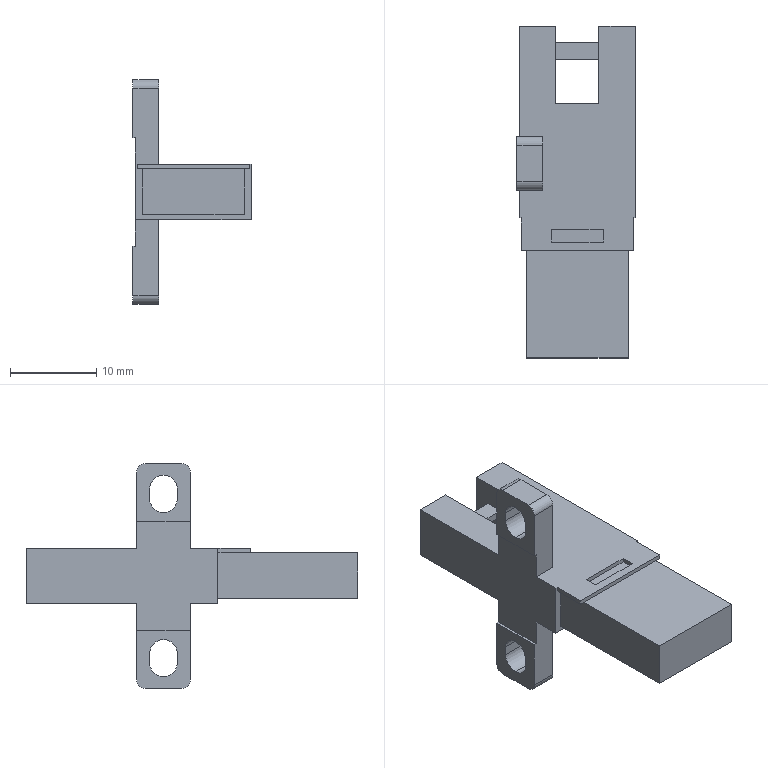Part | STEP file | Sensor EE-SX672_OMRON_default | 3 solids | 100 faces | box 13.7 x 38.4 x 26 mm | volume 2958 mm3 | plane 82 | cylinder 18 | commonest cylinder face diameters 0.8 x8 3.2 x6 2 x4